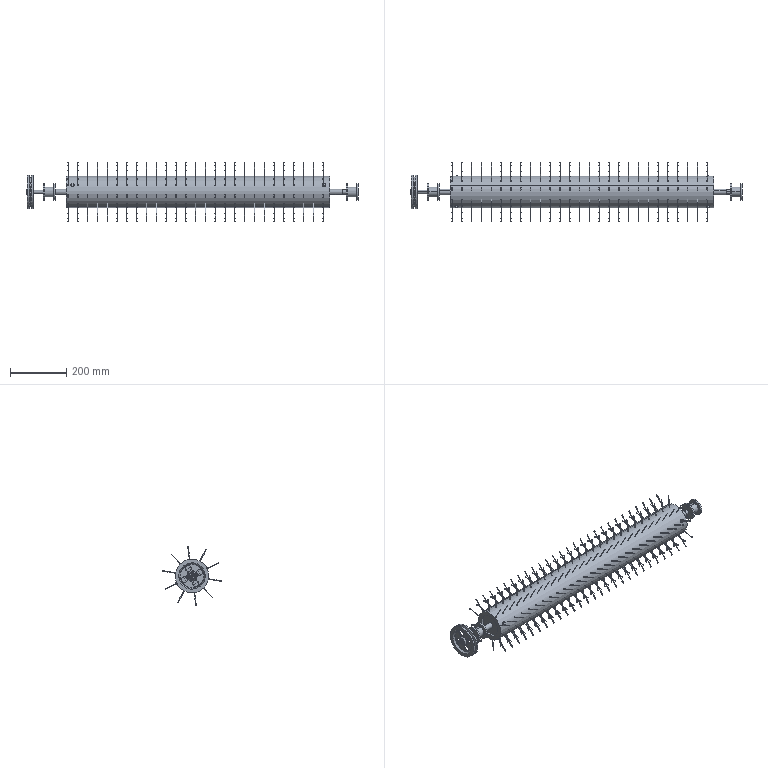Part | NX | features BREP 291 | 310 solids | 1452 faces | box 1184 x 209.075 x 210.255 mm | volume 5410753 mm3 | cylinder 747 | plane 675 | cone 22 | torus 8 | commonest cylinder face diameters 2 x538 6 x74 8 x32 12 x14 15 x12 19 x8